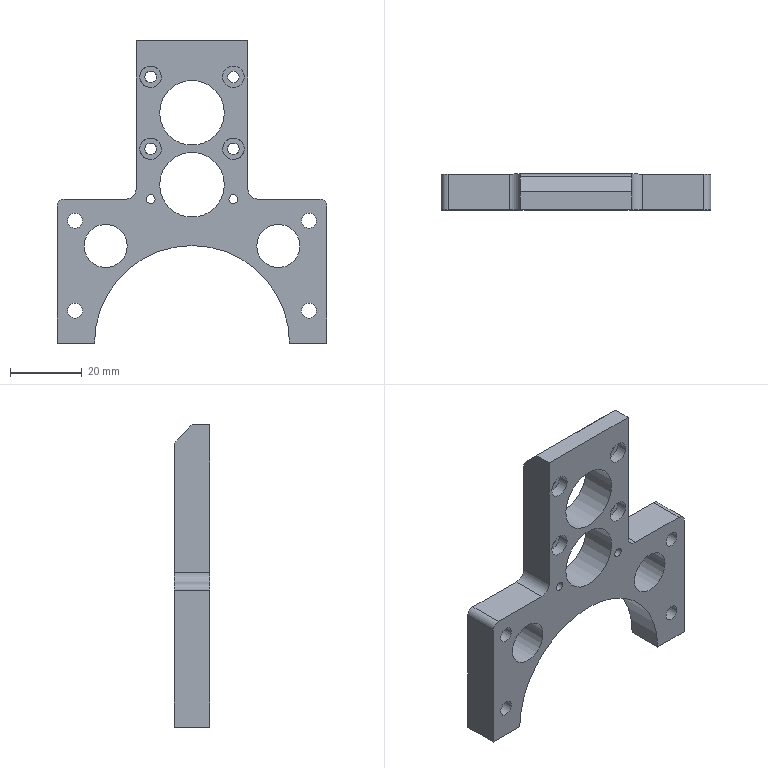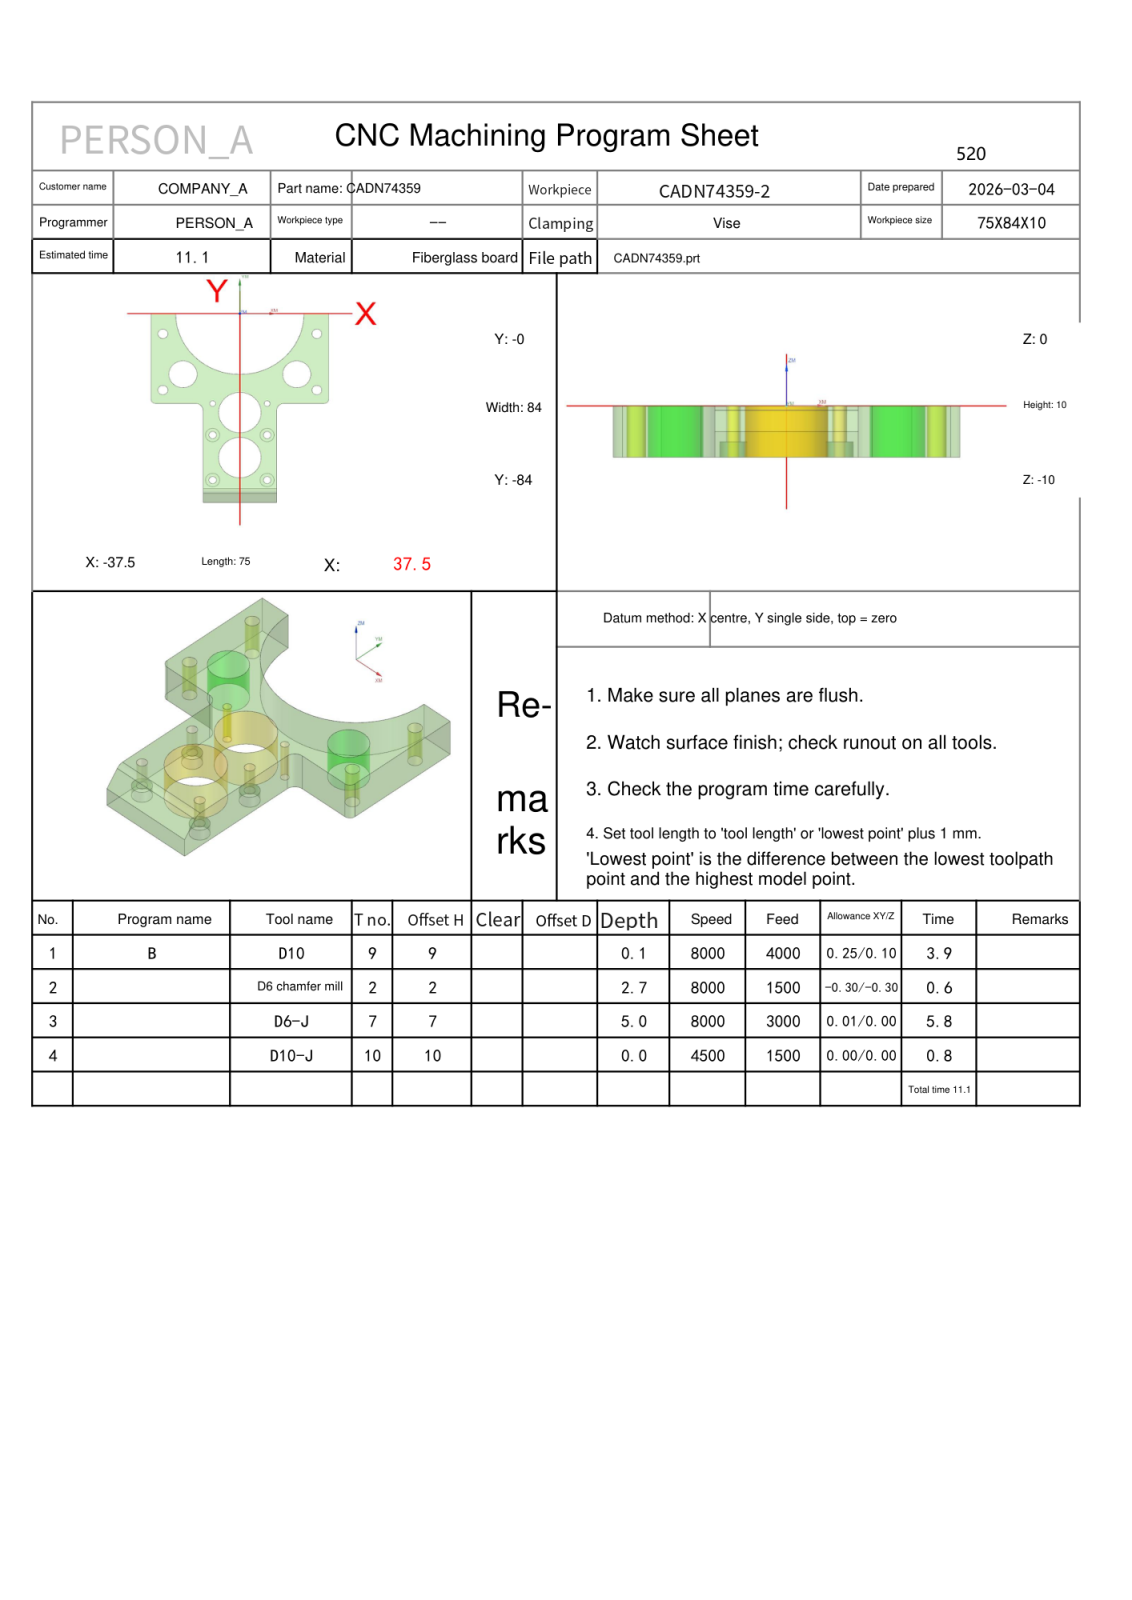NC program | NX | posted by the shop | part box 75 x 10 x 84 mm
Lines 1 to 788 of 5701:
%
O0001
(Machine time: 11.97 MIN)
(===Total Tool:4===)
(T9=D10     D=10.  R=0.   D-  H09 Z=0.1   )
(T2=D6 chamfer mill   D=6.   R=0.   D-  H02 Z=-2.7  )
(T7=D6-J    D=6.   R=0.   D-  H07 Z=-5.   )
(T10=D10-J  D=10.  R=0.   D-  H10 Z=-0.   )
G80 G90 G17 G49 G40
G91 G28 Z0
M01
N1 T09 M06
(D10  D=10. R=0. H=09 ce=0.25 di=0.10)
G00 G90 G54 X.981 Y-98.143 M03 S8000
G43 H09 Z50.
M08
Z2.1
G01 X.966 Y-98.044 Z1.476 F4000.
X.951 Y-97.946 Z1.228
X.936 Y-97.847 Z1.046
X.921 Y-97.748 Z.9
X.906 Y-97.649 Z.777
X.891 Y-97.55 Z.672
X.876 Y-97.451 Z.58
X.861 Y-97.352 Z.5
X.846 Y-97.253 Z.43
X.831 Y-97.155 Z.368
X.816 Y-97.056 Z.314
X.801 Y-96.957 Z.267
X.786 Y-96.858 Z.227
X.771 Y-96.759 Z.192
X.756 Y-96.66 Z.164
X.741 Y-96.561 Z.14
X.726 Y-96.463 Z.123
X.711 Y-96.364 Z.11
X.696 Y-96.265 Z.103
X.681 Y-96.166 Z.1
X.344 Y-93.943
G03 X-.025 Y-93.531 I-.502 J-.079
X-3.947 Y-93.062 I-3.922 J-16.183
X-4.192 Y-93.064 I0.0 J-16.651
X-12.906 Y-93.001 I-8.729 J-597.625
G01 X-38.606 Y-92.983
G02 X-45.538 Y-87.829 I.008 J7.25
X-46.404 Y-82.213 I19.028 J5.807
X-46.506 Y-73.24 I392.274 J8.973
X-46.5 Y-71.014 I392.377 J0.0
G01 X-46.482 Y1.105
G02 X-41.284 Y8.054 I7.259 J-.011
X-35.265 Y8.923 I6.019 J-20.415
G01 X-35.217
G02 X-25.629 Y9.001 I9.588 J-591.329
G01 X-24.568 Y9.
X38.569 Y8.984
X38.595
G02 X45.543 Y3.817 I0.0 J-7.254
X46.404 Y-1.799 I-19.128 J-5.808
X46.506 Y-10.786 I-395.917 J-8.987
X46.5 Y-12.997 I-396.019 J0.0
G01 X46.484 Y-85.069
Y-85.096
G02 X41.318 Y-92.042 I-7.254 J0.0
X35.454 Y-92.914 I-5.926 J19.698
X26.273 Y-93.003 I-9.181 J474.807
X24.505 Y-93. I0.0 J474.896
G01 X1.905 Y-92.983
G03 X-10.21 Y-92.487 I-12.115 J-147.947
X-12.258 Y-92.502 I0.0 J-148.443
G01 X-37.155 Y-92.483
G02 X-44.518 Y-87.498 I.03 J7.975
X-45.813 Y-81.465 I16.581 J6.714
X-46.005 Y-73.673 I158.093 J7.792
X-45.997 Y-72.119 I158.285 J0.0
G01 X-45.982 Y-.345
G02 X-41.109 Y6.968 I7.946 J-.015
X-35.088 Y8.304 I6.734 J-16.105
X-26.293 Y8.517 I8.795 J-181.694
X-23.742 Y8.499 I0.0 J-181.907
G01 X37.155 Y8.482
G02 X44.519 Y3.497 I-.03 J-7.976
X45.813 Y-2.536 I-16.585 J-6.714
X46.021 Y-11.891 I-211.085 J-9.356
X45.999 Y-14.882 I-211.292 J0.0
G01 X45.98 Y-83.705
G02 X40.998 Y-91.019 I-7.97 J.075
X34.965 Y-92.313 I-6.714 J16.583
X25.638 Y-92.52 I-9.327 J210.092
X22.669 Y-92.499 I0.0 J210.299
G01 X3.145 Y-92.481
G03 X-12.802 Y-91.996 I-15.948 J-261.611
X-14.355 Y-92. I0.0 J-262.097
G01 X-35.855 Y-91.98
G02 X-43.822 Y-86.659 I.07 J8.73
X-45.293 Y-80.005 I17.618 J7.384
X-45.511 Y-71.309 I173.46 J8.697
X-45.498 Y-69.159 I173.678 J0.0
G01 X-45.482 Y-1.709
G02 X-40.158 Y6.323 I8.737 J-.01
X-33.505 Y7.793 I7.384 J-17.621
X-24.516 Y8.014 I8.989 J-182.901
X-22.109 Y7.998 I0.0 J-183.122
G01 X35.791 Y7.982
G02 X43.822 Y2.658 I-.011 J-8.737
X45.293 Y-3.995 I-17.61 J-7.383
X45.505 Y-12.163 I-157.916 J-8.168
X45.497 Y-13.741 I-158.127 J0.0
G01 X45.482 Y-82.291
G02 X40.159 Y-90.322 I-8.736 J.01
X33.506 Y-91.793 I-7.383 J17.606
X24.547 Y-92.014 I-8.959 J181.875
X22.16 Y-91.998 I0.0 J182.095
G01 X4.06 Y-91.979
G03 X-8.259 Y-91.537 I-23.78 J-491.248
G01 X-14.806 Y-91.5
X-34.605 Y-91.477
G02 X-43.325 Y-85.538 I.045 J9.437
X-44.79 Y-78.574 I19.563 J7.751
X-45.017 Y-68.84 I208.452 J9.735
X-44.998 Y-66.028 I208.679 J0.0
G01 X-44.981 Y-3.028
X-44.982 Y-2.95
G02 X-39.038 Y5.826 I9.45 J0.0
X-32.073 Y7.29 I7.751 J-19.568
X-22.913 Y7.511 I9.161 J-189.555
X-20.627 Y7.498 I0.0 J-189.776
G01 X34.473 Y7.481
X34.555 Y7.482
G02 X43.305 Y1.584 I0.0 J-9.44
X44.764 Y-5.077 I-18.893 J-7.628
X45.005 Y-13.582 I-150.176 J-8.505
X44.996 Y-15.222 I-150.417 J0.0
G01 X44.976 Y-81.105
G02 X39.039 Y-89.825 I-9.437 J.044
X32.124 Y-91.287 I-7.726 J19.471
X22.834 Y-91.513 I-9.29 J190.343
X20.428 Y-91.498 I0.0 J190.57
X14.512 Y-91.52 I-5.917 J778.971
X3.379 Y-91.441 I0.0 J778.993
G03 X-14.966 Y-90.989 I-18.345 J-371.745
X-17.956 Y-91.001 I0.0 J-372.198
G02 X-23.739 Y-91.02 I-5.784 J870.958
X-33.655 Y-90.963 I0.0 J870.978
X-42.76 Y-84.669 I.167 J9.975
X-44.257 Y-77.709 I20.139 J7.971
X-44.503 Y-68.967 I154.81 J8.742
X-44.495 Y-67.364 I155.056 J0.0
G01 X-44.478 Y-4.214
X-44.479 Y-4.081
G02 X-41.71 Y2.875 I10.124 J0.0
X-35.255 Y6.189 I8.799 J-9.195
X-27.194 Y6.945 I8.061 J-42.605
G01 X-26.953 Y6.944
X-18.053 Y6.998
X33.247 Y6.979
X33.398 Y6.98
G02 X40.128 Y4.445 I0.0 J-10.2
X43.619 Y-1.943 I-8.622 J-8.86
X44.422 Y-9.638 I-37.618 J-7.815
X44.5 Y-19.696 I-649.557 J-10.058
X44.498 Y-21.137 I-649.635 J0.0
G01 X44.48 Y-79.737
X44.481 Y-79.894
G02 X41.95 Y-86.622 I-10.209 J0.0
X35.499 Y-90.133 I-8.884 J8.642
X27.524 Y-90.933 I-7.975 J39.351
G01 X27.453
G02 X15.821 Y-91.023 I-11.633 J748.006
X3.005 Y-90.914 I0.0 J748.096
G03 X-16.178 Y-90.486 I-19.182 J-430.123
X-19.653 Y-90.5 I0.0 J-430.551
G02 X-24.281 Y-90.522 I-4.628 J484.09
X-32.753 Y-90.448 I0.0 J484.112
X-42.196 Y-83.868 I.253 J10.429
X-43.737 Y-76.766 I20.807 J8.232
X-44.015 Y-66.782 I178.807 J9.984
X-43.997 Y-64.221 I179.085 J0.0
G01 X-43.978 Y-5.422
X-43.979 Y-5.258
G02 X-42.046 Y1.043 I11.234 J0.0
X-35.668 Y5.313 I9.395 J-7.134
X-28.061 Y6.37 I8.11 J-30.472
X-17.63 Y6.507 I10.431 J-395.168
X-14.912 Y6.498 I0.0 J-395.306
G01 X32.038 Y6.479
X32.217 Y6.48
G02 X38.385 Y4.657 I0.0 J-11.343
X42.772 Y-1.697 I-6.861 J-9.429
X43.868 Y-9.398 I-29.848 J-8.176
X44.008 Y-19.888 I-393.105 J-10.491
X43.998 Y-22.646 I-393.245 J0.0
G01 X43.975 Y-78.646
X43.976 Y-78.78
G02 X41.86 Y-85.295 I-11.085 J0.0
X35.324 Y-89.413 I-9.38 J7.642
X27.404 Y-90.395 I-8.195 J33.641
X15.088 Y-90.519 I-12.316 J614.848
X2.806 Y-90.396 I0.0 J614.972
G03 X-15.66 Y-89.998 I-18.465 J-428.124
X-17.156 Y-90.001 I0.0 J-428.522
G02 X-22.393 Y-90.022 I-5.237 J626.591
X-31.505 Y-89.956 I0.0 J626.612
X-38.708 Y-87.269 I.077 J11.204
X-42.477 Y-80.619 I8.965 J9.475
X-43.412 Y-72.187 I38.49 J8.534
X-43.5 Y-61.398 I662.317 J10.789
X-43.498 Y-59.838 I662.405 J0.0
G01 X-43.479 Y-6.638
G02 X-43.481 Y-6.409 I12.499 J.229
X-41.939 Y-.394 I12.501 J0.0
X-35.509 Y4.563 I9.862 J-6.145
X-27.835 Y5.824 I8.424 J-27.281
X-16.743 Y6.016 I11.093 J-320.128
X-13.338 Y5.998 I0.0 J-320.321
G01 X30.862 Y5.979
G02 X31.092 Y5.981 I.23 J-12.503
X37.101 Y4.442 I0.0 J-12.505
X42.063 Y-1.991 I-6.139 J-9.864
X43.318 Y-9.565 I-27.058 J-8.375
X43.517 Y-20.71 I-312.377 J-11.144
X43.498 Y-24.163 I-312.576 J0.0
G01 X43.479 Y-77.363
G02 X43.481 Y-77.591 I-12.502 J-.228
X41.939 Y-83.606 I-12.505 J0.0
X35.509 Y-88.563 I-9.859 J6.14
X27.935 Y-89.818 I-8.376 J27.064
X16.783 Y-90.017 I-11.152 J312.745
X13.338 Y-89.998 I0.0 J312.944
G01 X12.615 Y-89.999
G02 X-4.62 Y-89.639 I0.0 J412.949
G03 X-22.588 Y-89.476 I-17.968 J-991.376
X-28.856 Y-89.496 I0.0 J-991.538
G02 X-29.461 Y-89.506 I-.605 J17.101
X-34.623 Y-88.709 I0.0 J17.111
X-41.171 Y-82.175 I3.971 J10.527
X-42.731 Y-74.667 I22.968 J8.691
X-43.01 Y-64.586 I182.257 J10.082
X-42.995 Y-62.273 I182.536 J0.0
G01 X-42.973 Y-7.523
X-42.974 Y-7.357
G02 X-41.401 Y-1.137 I13.089 J0.0
X-34.874 Y3.977 I10.138 J-6.218
X-27.21 Y5.297 I8.595 J-26.985
X-15.524 Y5.52 I11.686 J-306.898
X-11.813 Y5.497 I0.0 J-307.12
G01 X29.737 Y5.479
G02 X30.001 Y5.482 I.265 J-13.775
X35.889 Y4.16 I0.0 J-13.777
X41.355 Y-2.29 I-5.538 J-10.233
X42.778 Y-9.981 I-25.381 J-8.673
X43.009 Y-20.085 I-221.256 J-10.104
X42.996 Y-22.427 I-221.487 J0.0
G01 X42.974 Y-76.427
X42.975 Y-76.612
G02 X41.451 Y-82.777 I-13.226 J0.0
X34.874 Y-87.977 I-10.173 J6.107
X26.961 Y-89.312 I-8.71 J27.512
X14.84 Y-89.521 I-12.121 J351.568
X10.713 Y-89.497 I0.0 J351.777
X-5.901 Y-89.112 I5.899 J613.846
G03 X-21.799 Y-88.977 I-15.899 J-933.696
X-27.756 Y-88.996 I0.0 J-933.831
G02 X-28.389 Y-89.006 I-.633 J18.902
X-33.587 Y-88.278 I0.0 J18.912
X-40.608 Y-81.501 I3.723 J10.882
X-42.205 Y-73.998 I23.112 J8.842
X-42.511 Y-63.662 I174.8 J10.336
X-42.495 Y-61.304 I175.106 J0.0
G01 X-42.477 Y-8.755
G02 X-42.48 Y-8.482 I14.679 J.272
X-41.2 Y-2.487 I14.682 J0.0
X-34.591 Y3.272 I10.533 J-5.416
X-26.709 Y4.764 I8.923 J-25.572
X-16.396 Y5.009 I10.313 J-217.484
X-14.013 Y4.996 I0.0 J-217.728
G01 X28.736 Y4.977
G02 X29.014 Y4.98 I.278 J-14.692
X35.005 Y3.704 I0.0 J-14.695
X40.781 Y-2.93 I-5.415 J-10.546
X42.256 Y-10.665 I-25.374 J-8.847
X42.507 Y-20.745 I-202.526 J-10.08
X42.495 Y-22.91 I-202.776 J0.0
G01 X42.471 Y-75.46
X42.472 Y-75.638
G02 X41.058 Y-81.794 I-14.102 J0.0
X34.395 Y-87.347 I-10.477 J5.798
X26.7 Y-88.765 I-8.796 J26.139
X16.408 Y-89.008 I-10.292 J217.44
X14.054 Y-88.996 I0.0 J217.683
X-5.108 Y-88.634 I.043 J510.252
G03 X-22.797 Y-88.476 I-17.688 J-988.713
X-27.405 Y-88.487 I0.0 J-988.871
G02 X-27.816 Y-88.492 I-.411 J17.095
X-33.541 Y-87.505 I0.0 J17.1
X-40.137 Y-80.635 I4.564 J10.982
X-41.738 Y-72.626 I24.973 J9.156
X-42.009 Y-62.149 I202.206 J10.476
X-41.995 Y-59.781 I202.478 J0.0
G01 X-41.975 Y-9.681
G02 X-41.977 Y-9.418 I15.521 J.262
X-40.741 Y-3.349 I15.523 J0.0
X-33.948 Y2.71 I10.829 J-5.303
X-26.125 Y4.238 I9.033 J-25.472
X-15.464 Y4.511 I10.661 J-208.007
X-12.93 Y4.495 I0.0 J-208.28
G01 X27.819 Y4.475
G02 X28.082 Y4.477 I.263 J-15.516
X34.152 Y3.241 I0.0 J-15.518
X40.21 Y-3.551 I-5.304 J-10.83
X41.738 Y-11.375 I-25.462 J-9.032
X42.01 Y-22.01 I-207.349 J-10.635
X41.995 Y-24.519 I-207.621 J0.0
G01 X41.975 Y-74.319
G02 X41.977 Y-74.569 I-15.629 J-.25
X40.783 Y-80.561 I-15.631 J0.0
X33.949 Y-86.711 I-10.859 J5.195
X26.076 Y-88.241 I-9.053 J25.553
X15.189 Y-88.513 I-10.887 J217.921
X12.381 Y-88.495 I0.0 J218.192
X-5.651 Y-88.125 I3.72 J620.899
G03 X-21.898 Y-87.979 I-16.247 J-902.114
X-26.256 Y-87.989 I0.0 J-902.261
G02 X-26.736 Y-87.995 I-.48 J19.236
X-32.371 Y-87.152 I0.0 J19.242
X-39.493 Y-80.213 I4.066 J11.298
X-41.189 Y-72.327 I23.942 J9.276
X-41.51 Y-61.594 I179.365 J10.733
X-41.494 Y-59.184 I179.686 J0.0
G01 X-41.47 Y-10.484
G02 X-41.471 Y-10.271 I16.044 J.214
X-40.218 Y-4.053 I16.046 J0.0
X-33.296 Y2.162 I11.056 J-5.351
X-25.229 Y3.735 I9.267 J-26.05
X-14.683 Y4.007 I10.546 J-204.458
X-12.384 Y3.994 I0.0 J-204.729
G01 X27.016 Y3.97
G02 X27.229 Y3.971 I.213 J-16.044
X33.448 Y2.717 I0.0 J-16.045
X39.663 Y-4.204 I-5.351 J-11.055
X41.236 Y-12.271 I-26.042 J-9.265
X41.507 Y-22.819 I-204.716 J-10.548
X41.494 Y-25.116 I-204.988 J0.0
G01 X41.47 Y-73.516
G02 X41.471 Y-73.729 I-16.051 J-.213
X40.218 Y-79.947 I-16.052 J0.0
X33.25 Y-86.181 I-11.069 J5.363
X25.229 Y-87.735 I-9.235 J26.173
X13.858 Y-88.015 I-11.372 J230.77
X10.184 Y-87.986 I0.0 J231.05
X-6.788 Y-87.604 I12.569 J935.853
G03 X-22.457 Y-87.476 I-15.669 J-960.257
X-25.706 Y-87.482 I0.0 J-960.385
G02 X-26.076 Y-87.486 I-.37 J18.449
X-32.094 Y-86.477 I0.0 J18.452
X-39.053 Y-79.318 I4.616 J11.449
X-40.711 Y-71.165 I25.601 J9.452
X-41.001 Y-61. I178.33 J10.165
X-40.992 Y-59.221 I178.62 J0.0
G01 X-40.974 Y-11.571
G02 X-40.976 Y-11.282 I17.598 J.289
X-39.874 Y-5.153 I17.6 J0.0
X-32.817 Y1.553 I11.36 J-4.888
X-24.665 Y3.211 I9.453 J-25.605
X-13.487 Y3.512 I11.178 J-207.246
X-10.771 Y3.495 I0.0 J-207.547
G01 X25.929 Y3.473
G02 X26.218 Y3.476 I.289 J-17.596
X32.347 Y2.374 I0.0 J-17.599
X39.053 Y-4.683 I-4.888 J-11.36
X40.711 Y-12.835 I-25.597 J-9.451
X41.003 Y-23.18 I-183.457 J-10.345
X40.992 Y-25.13 I-183.748 J0.0
G01 X40.973 Y-72.429
G02 X40.976 Y-72.715 I-17.619 J-.286
X39.874 Y-78.847 I-17.622 J0.0
X32.818 Y-85.553 I-11.359 J4.888
X24.665 Y-87.211 I-9.453 J25.606
X13.409 Y-87.512 I-11.255 J210.223
X9.62 Y-87.478 I0.0 J210.524
X-6.291 Y-87.117 I12.284 J891.287
G03 X-22.237 Y-86.978 I-15.946 J-915.117
X-24.806 Y-86.982 I0.0 J-915.256
G02 X-25.181 Y-86.985 I-.375 J19.522
X-31.253 Y-86.017 I0.0 J19.526
X-38.414 Y-78.921 I4.435 J11.637
X-40.18 Y-70.694 I24.843 J9.638
X-40.497 Y-60.555 I161.932 J10.139
X-40.49 Y-58.951 I162.249 J0.0
G01 X-40.48 Y-12.801
G02 X-40.484 Y-12.383 I20.028 J.418
X-39.568 Y-6.395 I20.033 J0.0
X-32.421 Y.913 I11.677 J-4.271
X-24.194 Y2.68 I9.638 J-24.84
X-13.981 Y2.998 I10.213 J-163.729
X-12.301 Y2.99 I0.0 J-164.047
G01 X24.699 Y2.979
G02 X25.117 Y2.984 I.418 J-20.027
X31.106 Y2.068 I0.0 J-20.031
X38.414 Y-5.079 I-4.271 J-11.677
X40.159 Y-13.057 I-24.413 J-9.522
X40.496 Y-23.171 I-151.696 J-10.114
X40.488 Y-24.699 I-152.033 J0.0
G01 X40.479 Y-71.199
G02 X40.484 Y-71.618 I-20.029 J-.419
X39.568 Y-77.605 I-20.034 J0.0
X32.46 Y-84.897 I-11.67 J4.264
X24.382 Y-86.665 I-9.579 J24.435
X13.391 Y-87.008 I-10.991 J175.929
X10.09 Y-86.977 I0.0 J176.272
X-6.092 Y-86.623 I10.834 J866.587
G03 X-21.82 Y-86.479 I-15.728 J-857.992
X-23.907 Y-86.482 I0.0 J-858.136
G02 X-24.303 Y-86.485 I-.395 J20.58
X-30.461 Y-85.543 I0.0 J20.583
X-37.904 Y-78.231 I4.357 J11.88
X-39.661 Y-70.1 I25.1 J9.678
X-39.996 Y-59.886 I155.548 J10.214
X-39.988 Y-58.358 I155.883 J0.0
G01 X-39.971 Y-13.308
G02 X-39.974 Y-13.01 I19.341 J.298
X-38.924 Y-6.725 I19.343 J0.0
X-31.731 Y.403 I11.774 J-4.687
X-23.6 Y2.16 I9.678 J-25.094
X-12.689 Y2.505 I10.911 J-172.51
X-10.508 Y2.491 I0.0 J-172.854
G01 X24.142 Y2.472
G02 X24.441 Y2.474 I.298 J-19.758
X30.588 Y1.494 I0.0 J-19.76
X37.903 Y-5.769 I-4.484 J-11.833
X39.665 Y-13.95 I-25.174 J-9.7
X40.005 Y-24.829 I-173.917 J-10.88
X39.991 Y-26.992 I-174.257 J0.0
G01 X39.972 Y-70.642
G02 X39.974 Y-70.941 I-19.762 J-.299
X38.994 Y-77.088 I-19.764 J0.0
X31.732 Y-84.403 I-11.833 J4.485
X23.599 Y-86.161 I-9.678 J25.091
X12.665 Y-86.503 I-10.934 J174.587
X8.856 Y-86.461 I0.0 J174.929
X-6.091 Y-86.125 I12.238 J877.39
G03 X-21.792 Y-85.979 I-15.701 J-844.664
X-23.109 Y-85.98 I0.0 J-844.81
G02 X-23.496 Y-85.984 I-.387 J21.239
X-29.764 Y-85.038 I0.0 J21.242
X-37.366 Y-77.621 I4.349 J12.062
X-39.143 Y-69.497 I25.206 J9.769
X-39.499 Y-58.836 I159.202 J10.661
X-39.489 Y-57.005 I159.559 J0.0
G01 X-39.472 Y-14.205
G02 X-39.474 Y-13.886 I20.517 J.319
X-38.49 Y-7.609 I20.52 J0.0
X-31.213 Y-.174 I11.996 J-4.463
X-22.997 Y1.643 I9.828 J-24.967
X-12.554 Y1.996 I10.443 J-154.225
X-10.955 Y1.988 I0.0 J-154.578
G01 X23.295 Y1.971
G02 X23.614 Y1.974 I.32 J-20.522
X29.891 Y.99 I0.0 J-20.525
X37.326 Y-6.287 I-4.462 J-11.996
X39.143 Y-14.503 I-24.962 J-9.828
X39.496 Y-24.941 I-154.138 J-10.438
X39.487 Y-26.545 I-154.491 J0.0
G01 X39.471 Y-69.794
G02 X39.474 Y-70.115 I-20.52 J-.321
X38.491 Y-76.391 I-20.522 J0.0
X31.214 Y-83.826 I-11.996 J4.462
X22.998 Y-85.643 I-9.828 J24.964
X12.185 Y-85.996 I-10.812 J165.177
X8.206 Y-85.948 I0.0 J165.53
G01 X-9.513 Y-85.57
X-22.963 Y-85.463
X-23.085 Y-85.464
G02 X-29.632 Y-84.33 I0.0 J19.468
X-36.894 Y-76.865 I4.961 J12.091
X-38.654 Y-68.576 I26.197 J9.893
X-39.008 Y-57.035 I187.753 J11.541
X-38.992 Y-54.534 I188.108 J0.0
G01 X-38.971 Y-15.034
G02 X-38.973 Y-14.713 I21.448 J.321
X-38.017 Y-8.38 I21.45 J0.0
X-30.543 Y-.681 I12.21 J-4.376
X-22.176 Y1.145 I9.966 J-25.575
X-10.964 Y1.505 I11.211 J-174.716
X-8.734 Y1.49 I0.0 J-175.076
G01 X22.466 Y1.471
G02 X22.788 Y1.473 I.322 J-21.451
X29.12 Y.517 I0.0 J-21.454
X36.819 Y-6.957 I-4.376 J-12.21
X38.646 Y-15.324 I-25.572 J-9.965
X39.005 Y-26.541 I-175.03 J-11.217
X38.99 Y-28.766 I-175.389 J0.0
G01 X38.971 Y-68.966
G02 X38.973 Y-69.289 I-21.447 J-.323
X38.017 Y-75.62 I-21.449 J0.0
X30.544 Y-83.319 I-12.209 J4.376
X22.176 Y-85.145 I-9.966 J25.574
X11.54 Y-85.488 I-10.636 J165.13
X7.084 Y-85.428 I0.0 J165.472
G01 X-9.81 Y-85.068
G02 X-22.966 Y-84.933 I2.275 J862.519
X-29.902 Y-83.417 I.174 J17.425
X-36.462 Y-76.018 I6.062 J11.981
X-38.157 Y-67.768 I27.284 J9.905
X-38.501 Y-56.672 I178.543 J11.096
X-38.49 Y-54.626 I178.887 J0.0
G01 X-38.468 Y-15.726
G02 X-38.469 Y-15.455 I21.918 J.271
X-37.519 Y-9.07 I21.919 J0.0
X-29.981 Y-1.229 I12.369 J-4.347
X-21.766 Y.613 I9.987 J-25.296
X-10.851 Y.998 I10.915 J-154.573
X-9.025 Y.987 I0.0 J-154.958
G01 X21.774 Y.967
G02 X22.046 Y.969 I.272 J-21.918
X28.43 Y.019 I0.0 J-21.919
X36.271 Y-7.519 I-4.347 J-12.368
X38.113 Y-15.734 I-25.293 J-9.987
X38.493 Y-26.349 I-148.143 J-10.615
X38.485 Y-27.875 I-148.523 J0.0
G01 X38.478 Y-67.724
G02 X38.483 Y-68.213 I-24.369 J-.489
X37.658 Y-74.502 I-24.374 J0.0
X29.981 Y-82.771 I-12.495 J3.902
X21.767 Y-84.613 I-9.986 J25.291
X11.348 Y-84.979 I-10.419 J148.296
X7.426 Y-84.927 I0.0 J148.662
G01 X-10.804 Y-84.557
X-10.843
G02 X-22.469 Y-84.42 I0.0 J492.104
X-29.571 Y-82.756 I.278 J17.179
X-35.982 Y-75.296 I6.461 J12.036
X-37.674 Y-66.79 I28.361 J10.063
X-38.009 Y-54.904 I210.618 J11.886
X-37.992 Y-52.197 I210.954 J0.0
G01 X-37.971 Y-16.697
G02 X-37.973 Y-16.357 I23.603 J.34
X-37.095 Y-9.978 I23.605 J0.0
X-29.294 Y-1.72 I12.615 J-4.103
X-20.729 Y.138 I10.2 J-26.344
X-9.418 Y.502 I11.311 J-175.592
X-7.288 Y.489 I0.0 J-175.956
G01 X20.762 Y.471
G02 X21.117 Y.474 I.355 J-23.798
X27.483 Y-.393 I0.0 J-23.801
X35.78 Y-8.206 I-4.063 J-12.626
X37.638 Y-16.771 I-26.338 J-10.198
X37.994 Y-27.487 I-161.396 J-10.716
X37.986 Y-29.062 I-161.751 J0.0
G01 X37.971 Y-67.262
G02 X37.974 Y-67.618 I-23.801 J-.356
X37.107 Y-73.983 I-23.804 J0.0
X29.295 Y-82.28 I-12.626 J4.062
X20.73 Y-84.138 I-10.194 J26.326
X10.502 Y-84.467 I-10.228 J158.517
X5.688 Y-84.394 I0.0 J158.847
G03 X-19.675 Y-83.987 I-28.532 J-987.644
G02 X-20.116 Y-83.991 I-.441 J26.24
X-26.557 Y-83.188 I0.0 J26.243
X-35.237 Y-75.24 I3.784 J12.846
X-37.094 Y-66.974 I25.846 J10.148
X-37.496 Y-55.895 I152.733 J11.079
X-37.486 Y-54.134 I153.134 J0.0
G01 X-37.469 Y-17.434
G02 X-37.472 Y-17.089 I24.015 J.345
X-36.57 Y-10.568 I24.018 J0.0
X-28.74 Y-2.263 I12.731 J-4.16
X-20.524 Y-.411 I10.124 J-25.75
X-9.691 Y-.009 I10.833 J-145.803
X-8.185 Y-.016 I0.0 J-146.205
G01 X20.015 Y-.03
G02 X20.381 Y-.027 I.365 J-24.248
X26.884 Y-.916 I0.0 J-24.251
X35.237 Y-8.76 I-4.11 J-12.746
X37.09 Y-16.976 I-25.742 J-10.122
X37.5 Y-28.315 I-156.631 J-11.339
X37.487 Y-30.316 I-157.041 J0.0
G01 X37.47 Y-66.515
G02 X37.473 Y-66.88 I-24.259 J-.364
X36.585 Y-73.384 I-24.262 J0.0
X28.74 Y-81.737 I-12.745 J4.11
X20.275 Y-83.612 I-10.224 J26.111
X10.118 Y-83.958 I-10.158 J148.974
X5.484 Y-83.886 I0.0 J149.32
G03 X-19.029 Y-83.487 I-28.473 J-997.013
G02 X-19.412 Y-83.49 I-.383 J26.6
X-25.912 Y-82.684 I0.0 J26.603
X-34.727 Y-74.617 I3.793 J12.995
X-36.607 Y-66.107 I26.469 J10.312
X-36.992 Y-55.145 I155.846 J10.962
X-36.984 Y-53.566 I156.231 J0.0
G01 X-36.969 Y-18.216
G02 X-36.972 Y-17.849 I24.779 J.367
X-36.076 Y-11.248 I24.781 J0.0
X-28.117 Y-2.774 I12.887 J-4.13
X-19.607 Y-.893 I10.312 J-26.459
X-7.968 Y-.498 I11.638 J-171.22
X-5.766 Y-.512 I0.0 J-171.615
G01 X19.084 Y-.528
G02 X19.518 Y-.524 I.434 J-25.847
X26.061 Y-1.366 I0.0 J-25.85
X34.726 Y-9.382 I-3.935 J-12.945
X36.607 Y-17.893 I-26.451 J-10.31
X37.002 Y-29.51 I-170.842 J-11.617
X36.988 Y-31.684 I-171.237 J0.0
G01 X36.973 Y-65.534
G02 X36.977 Y-65.997 I-25.978 J-.463
X36.135 Y-72.561 I-25.982 J0.0
X28.118 Y-81.226 I-12.944 J3.935
X19.656 Y-83.101 I-10.271 J26.318
X9.565 Y-83.446 I-10.091 J147.365
X4.765 Y-83.368 I0.0 J147.71
G03 X-18.684 Y-82.981 I-27.869 J-977.746
G02 X-18.925 Y-82.982 I-.241 J25.188
X-25.603 Y-82.081 I0.0 J25.19
X-34.186 Y-74.072 I4.116 J13.015
X-36.096 Y-65.513 I26.503 J10.406
X-36.5 Y-53.873 I167.473 J11.64
X-36.487 Y-51.773 I167.877 J0.0
G01 X-36.473 Y-19.223
G02 X-36.476 Y-18.788 I27.271 J.435
X-35.69 Y-12.287 I27.274 J0.0
X-27.572 Y-3.315 I13.116 J-3.708
X-18.868 Y-1.391 I10.473 J-26.735
X-7.199 Y-.999 I11.669 J-173.474
X-5.028 Y-1.013 I0.0 J-173.866
G01 X18.672 Y-1.035
G02 X18.962 Y-1.033 I.289 J-25.215
X25.545 Y-1.908 I0.0 J-25.216
X34.185 Y-9.928 I-4.045 J-13.022
X36.109 Y-18.632 I-26.726 J-10.471
X36.501 Y-30.279 I-173.044 J-11.647
X36.487 Y-32.423 I-173.435 J0.0
G01 X36.474 Y-64.722
G02 X36.477 Y-65.175 I-27.596 J-.453
X35.705 Y-71.661 I-27.6 J0.0
X27.573 Y-80.685 I-13.13 J3.655
X18.919 Y-82.601 I-10.413 J26.527
X9.14 Y-82.933 I-9.779 J144.128
X4.527 Y-82.859 I0.0 J144.46
G03 X-18.089 Y-82.481 I-27.925 J-992.358
G01 X-18.281
G02 X-25.101 Y-81.537 I0.0 J25.1
X-33.6 Y-73.639 I4.221 J13.064
X-35.549 Y-65.297 I25.703 J10.403
X-35.983 Y-54.438 I135.666 J10.858
X-35.978 Y-53.259 I136.1 J0.0
G01 X-35.973 Y-20.009
G02 X-35.977 Y-19.557 I28.37 J.452
X-35.213 Y-13.019 I28.373 J0.0
X-27.015 Y-3.847 I13.265 J-3.607
X-18.411 Y-1.914 I10.49 J-26.576
X-7.385 Y-1.511 I11.026 J-150.889
X-5.921 Y-1.518 I0.0 J-151.291
G01 X17.529 Y-1.528
G02 X17.987 Y-1.524 I.458 J-27.829
X24.614 Y-2.324 I0.0 J-27.833
X33.594 Y-10.347 I-3.716 J-13.196
X35.543 Y-18.641 I-25.565 J-10.383
X35.991 Y-29.915 I-141.735 J-11.274
X35.981 Y-31.529 I-142.183 J0.0
G01 X35.972 Y-64.029
G02 X35.976 Y-64.487 I-27.834 J-.458
X35.176 Y-71.114 I-27.838 J0.0
X27.153 Y-80.094 I-13.195 J3.715
X18.46 Y-82.077 I-10.516 J26.047
X8.883 Y-82.42 I-9.577 J133.62
X4.869 Y-82.36 I0.0 J133.963
G03 X-15.744 Y-82.015 I-26.948 J-995.125
G02 X-16.355 Y-82.02 I-.611 J37.642
X-22.91 Y-81.445 I0.0 J37.647
X-33.148 Y-72.904 I2.701 J13.644
X-35.054 Y-64.55 I26.435 J10.428
X-35.493 Y-53.046 I150.547 J11.504
X-35.483 Y-51.261 I150.986 J0.0
G01 X-35.473 Y-20.761
G02 X-35.477 Y-20.278 I28.968 J.484
X-34.702 Y-13.622 I28.972 J0.0
X-26.466 Y-4.38 I13.367 J-3.621
X-17.915 Y-2.433 I10.528 J-26.485
X-6.374 Y-2.005 I11.541 J-155.731
X-4.526 Y-2.016 I0.0 J-156.158
G01 X16.974 Y-2.031
G02 X17.351 Y-2.029 I.378 J-27.899
X24.008 Y-2.835 I0.0 J-27.902
X33.121 Y-11.034 I-3.75 J-13.33
X35.068 Y-19.585 I-26.473 J-10.525
X35.494 Y-31.077 I-154.742 J-11.492
X35.483 Y-32.874 I-155.168 J0.0
G01 X35.473 Y-63.224
G02 X35.477 Y-63.705 I-29.129 J-.48
X34.705 Y-70.364 I-29.133 J0.0
X26.466 Y-79.62 I-13.369 J3.605
X17.865 Y-81.566 I-10.488 J26.384
X8.43 Y-81.907 I-9.435 J130.318
X4.574 Y-81.85 I0.0 J130.659
G03 X-14.898 Y-81.522 I-26.46 J-994.599
G02 X-15.529 Y-81.527 I-.631 J39.455
X-22.215 Y-80.957 I0.0 J39.46
X-32.667 Y-72.239 I2.645 J13.796
X-34.563 Y-63.78 I27.067 J10.508
X-34.996 Y-51.983 I160.192 J11.798
X-34.984 Y-49.991 I160.625 J0.0
G01 X-34.965 Y-21.091
G02 X-34.967 Y-20.731 I27.376 J.36
X-34.105 Y-13.915 I27.378 J0.0
X-25.821 Y-4.869 I13.403 J-3.959
X-17.172 Y-2.927 I10.608 J-27.008
X-5.604 Y-2.506 I11.568 J-158.881
X-3.782 Y-2.517 I0.0 J-159.301
G01 X16.418 Y-2.535
G02 X16.745 Y-2.533 I.327 J-27.679
X23.498 Y-3.37 I0.0 J-27.681
X32.641 Y-11.702 I-3.877 J-13.437
X34.571 Y-20.305 I-27.019 J-10.579
X34.989 Y-31.6 I-152.382 J-11.295
X34.981 Y-33.144 I-152.8 J0.0
G01 X34.969 Y-62.694
G02 X34.972 Y-63.101 I-28.955 J-.407
X34.191 Y-69.782 I-28.958 J0.0
X25.798 Y-79.14 I-13.49 J3.656
X16.995 Y-81.079 I-10.581 J27.094
X7.489 Y-81.393 I-9.506 J143.584
X2.703 Y-81.314 I0.0 J143.898
G01 X-17.051 Y-80.955
G02 X-24.114 Y-79.73 I.237 J22.346
X-32.103 Y-71.776 I5.148 J13.16
X-34.056 Y-63.178 I26.958 J10.643
X-34.494 Y-51.455 I156.627 J11.723
X-34.483 Y-49.589 I157.065 J0.0
G01 X-34.467 Y-21.94
G02 X-34.47 Y-21.519 I28.645 J.421
X-33.625 Y-14.609 I28.648 J0.0
X-25.371 Y-5.439 I13.508 J-3.859
X-16.732 Y-3.45 I10.68 J-26.622
X-5.156 Y-3.009 I11.575 J-151.842
X-3.443 Y-3.019 I0.0 J-152.282
X4.315 Y-2.986 I7.758 J-916.499
X17.056 Y-3.074 I0.0 J-916.532
X24.171 Y-4.303 I-.132 J-21.974
X32.159 Y-12.359 I-5.221 J-13.164
X34.079 Y-21.067 I-27.636 J-10.658
X34.493 Y-32.694 I-162.933 J-11.627
X34.483 Y-34.507 I-163.348 J0.0
G01 X34.469 Y-61.957
G02 X34.472 Y-62.403 I-29.414 J-.446
X33.666 Y-69.243 I-29.417 J0.0
X25.37 Y-78.56 I-13.544 J3.707
X16.83 Y-80.528 I-10.537 J26.214
X7.388 Y-80.881 I-9.442 J126.045
X3.54 Y-80.823 I0.0 J126.398
G01 X-15.956 Y-80.476
G02 X-23.237 Y-79.329 I.077 J24.17
X-31.588 Y-71.205 I4.861 J13.35
X-33.57 Y-62.36 I27.484 J10.804
X-33.986 Y-51.035 I153.982 J11.325
X-33.979 Y-49.62 I154.398 J0.0
G01 X-33.967 Y-22.67
G02 X-33.97 Y-22.232 I29.448 J.438
X-33.14 Y-15.287 I29.452 J0.0
X-24.706 Y-5.915 I13.645 J-3.798
X-16.11 Y-3.954 I10.688 J-27.029
X-4.427 Y-3.509 I11.684 J-153.042
X-2.672 Y-3.519 I0.0 J-153.487
X4.382 Y-3.49 I7.053 J-854.12
X16.328 Y-3.573 I0.0 J-854.149
X23.541 Y-4.796 I-.104 J-22.507
X31.585 Y-12.794 I-5.161 J-13.234
X33.569 Y-21.639 I-27.424 J-10.798
X33.989 Y-33.159 I-157.921 J-11.52
X33.981 Y-34.779 I-158.341 J0.0
G01 X33.967 Y-61.328
G02 X33.97 Y-61.745 I-29.767 J-.417
X33.167 Y-68.615 I-29.77 J0.0
X24.705 Y-78.084 I-13.666 J3.697
X15.706 Y-80.065 I-10.737 J27.346
X6.696 Y-80.364 I-9.01 J135.67
X2.664 Y-80.304 I0.0 J135.969
G01 X-15.31 Y-79.98
G02 X-22.593 Y-78.844 I.112 J24.632
X-31.115 Y-70.535 I4.847 J13.496
X-33.053 Y-61.879 I27.674 J10.739
X-33.489 Y-50.214 I155.646 J11.665
X-33.48 Y-48.54 I156.083 J0.0
G01 X-33.467 Y-23.391
G02 X-33.47 Y-22.963 I30.603 J.427
X-32.679 Y-16.051 I30.606 J0.0
X-24.268 Y-6.486 I13.756 J-3.616